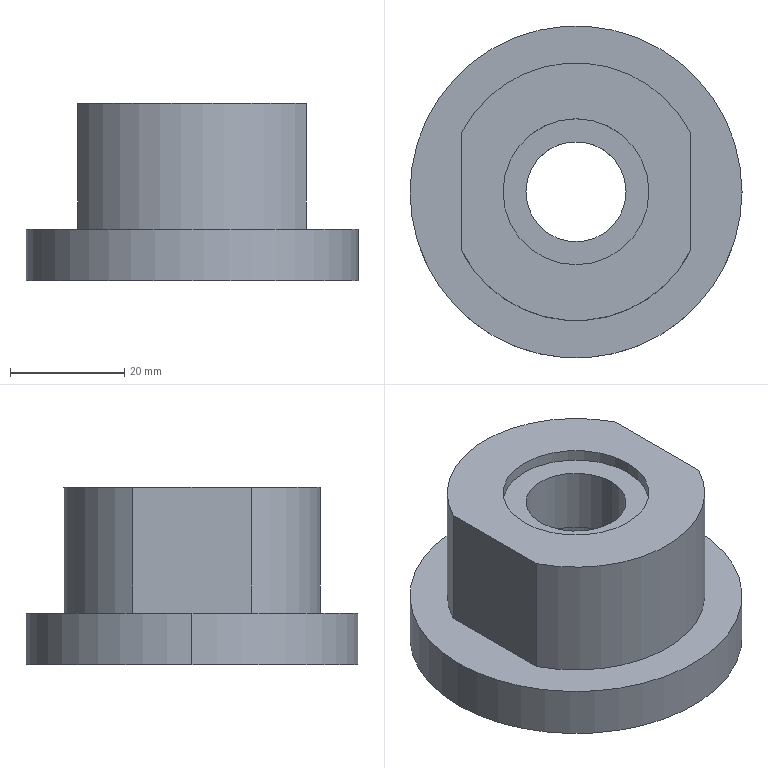Part | SolidWorks | features BaseBody 1 | 1 solid | 17 faces | box 58 x 58 x 31 mm | volume 44160 mm3 | cylinder 10 | plane 7 | commonest cylinder face diameters 17.5 x2 25.5 x2 26 x2 45 x2 58 x2
STEP:
#1=CARTESIAN_POINT('',(13.,0.,17.5));
#2=VERTEX_POINT('',#1);
#3=CARTESIAN_POINT('',(-13.,0.,17.5));
#4=VERTEX_POINT('',#3);
#5=CARTESIAN_POINT('',(0.,0.,17.5));
#6=DIRECTION('',(0.,0.,-1.));
#7=DIRECTION('',(-1.,0.,0.));
#8=AXIS2_PLACEMENT_3D('',#5,#6,#7);
#9=CIRCLE('',#8,13.);
#10=EDGE_CURVE('',#2,#4,#9,.T.);
#11=ORIENTED_EDGE('',*,*,#10,.F.);
#12=CARTESIAN_POINT('',(13.,0.,0.));
#13=VERTEX_POINT('',#12);
#14=CARTESIAN_POINT('',(13.,0.,0.));
#15=DIRECTION('',(0.,0.,-1.));
#16=VECTOR('',#15,1000.);
#17=LINE('',#14,#16);
#18=EDGE_CURVE('',#2,#13,#17,.T.);
#19=ORIENTED_EDGE('',*,*,#18,.T.);
#20=CARTESIAN_POINT('',(-13.,0.,0.));
#21=VERTEX_POINT('',#20);
#22=CARTESIAN_POINT('',(0.,0.,0.));
#23=DIRECTION('',(0.,0.,-1.));
#24=DIRECTION('',(-1.,0.,0.));
#25=AXIS2_PLACEMENT_3D('',#22,#23,#24);
#26=CIRCLE('',#25,13.);
#27=EDGE_CURVE('',#13,#21,#26,.T.);
#28=ORIENTED_EDGE('',*,*,#27,.T.);
#29=CARTESIAN_POINT('',(-13.,0.,0.));
#30=DIRECTION('',(0.,0.,-1.));
#31=VECTOR('',#30,1000.);
#32=LINE('',#29,#31);
#33=EDGE_CURVE('',#4,#21,#32,.T.);
#34=ORIENTED_EDGE('',*,*,#33,.F.);
#35=EDGE_LOOP('',(#11,#19,#28,#34));
#36=FACE_OUTER_BOUND('',#35,.T.);
#37=CARTESIAN_POINT('',(0.,0.,0.));
#38=DIRECTION('',(0.,0.,-1.));
#39=DIRECTION('',(-1.,0.,0.));
#40=AXIS2_PLACEMENT_3D('',#37,#38,#39);
#41=CYLINDRICAL_SURFACE('',#40,13.);
#42=ADVANCED_FACE('',(#36),#41,.F.);
#43=CARTESIAN_POINT('',(-8.75,0.,29.));
#44=VERTEX_POINT('',#43);
#45=CARTESIAN_POINT('',(8.75,0.,29.));
#46=VERTEX_POINT('',#45);
#47=CARTESIAN_POINT('',(0.,0.,29.));
#48=DIRECTION('',(0.,0.,1.));
#49=DIRECTION('',(1.,0.,0.));
#50=AXIS2_PLACEMENT_3D('',#47,#48,#49);
#51=CIRCLE('',#50,8.75);
#52=EDGE_CURVE('',#44,#46,#51,.T.);
#53=ORIENTED_EDGE('',*,*,#52,.T.);
#54=CARTESIAN_POINT('',(8.75,0.,17.5));
#55=VERTEX_POINT('',#54);
#56=CARTESIAN_POINT('',(8.75,0.,0.));
#57=DIRECTION('',(0.,0.,-1.));
#58=VECTOR('',#57,1000.);
#59=LINE('',#56,#58);
#60=EDGE_CURVE('',#46,#55,#59,.T.);
#61=ORIENTED_EDGE('',*,*,#60,.T.);
#62=CARTESIAN_POINT('',(-8.75,0.,17.5));
#63=VERTEX_POINT('',#62);
#64=CARTESIAN_POINT('',(0.,0.,17.5));
#65=DIRECTION('',(0.,0.,-1.));
#66=DIRECTION('',(-1.,0.,0.));
#67=AXIS2_PLACEMENT_3D('',#64,#65,#66);
#68=CIRCLE('',#67,8.75);
#69=EDGE_CURVE('',#55,#63,#68,.T.);
#70=ORIENTED_EDGE('',*,*,#69,.T.);
#71=CARTESIAN_POINT('',(-8.75,0.,0.));
#72=DIRECTION('',(0.,0.,-1.));
#73=VECTOR('',#72,1000.);
#74=LINE('',#71,#73);
#75=EDGE_CURVE('',#44,#63,#74,.T.);
#76=ORIENTED_EDGE('',*,*,#75,.F.);
#77=EDGE_LOOP('',(#53,#61,#70,#76));
#78=FACE_OUTER_BOUND('',#77,.T.);
#79=CARTESIAN_POINT('',(0.,0.,0.));
#80=DIRECTION('',(0.,0.,-1.));
#81=DIRECTION('',(-1.,0.,0.));
#82=AXIS2_PLACEMENT_3D('',#79,#80,#81);
#83=CYLINDRICAL_SURFACE('',#82,8.75);
#84=ADVANCED_FACE('',(#78),#83,.F.);
#85=CARTESIAN_POINT('',(-12.75,0.,29.));
#86=VERTEX_POINT('',#85);
#87=CARTESIAN_POINT('',(12.75,0.,29.));
#88=VERTEX_POINT('',#87);
#89=CARTESIAN_POINT('',(0.,0.,29.));
#90=DIRECTION('',(0.,0.,1.));
#91=DIRECTION('',(1.,0.,0.));
#92=AXIS2_PLACEMENT_3D('',#89,#90,#91);
#93=CIRCLE('',#92,12.75);
#94=EDGE_CURVE('',#86,#88,#93,.T.);
#95=ORIENTED_EDGE('',*,*,#94,.F.);
#96=CARTESIAN_POINT('',(-12.75,0.,31.));
#97=VERTEX_POINT('',#96);
#98=CARTESIAN_POINT('',(-12.75,0.,29.));
#99=DIRECTION('',(0.,0.,1.));
#100=VECTOR('',#99,1000.);
#101=LINE('',#98,#100);
#102=EDGE_CURVE('',#86,#97,#101,.T.);
#103=ORIENTED_EDGE('',*,*,#102,.T.);
#104=CARTESIAN_POINT('',(12.75,0.,31.));
#105=VERTEX_POINT('',#104);
#106=CARTESIAN_POINT('',(0.,0.,31.));
#107=DIRECTION('',(0.,0.,1.));
#108=DIRECTION('',(1.,0.,0.));
#109=AXIS2_PLACEMENT_3D('',#106,#107,#108);
#110=CIRCLE('',#109,12.75);
#111=EDGE_CURVE('',#97,#105,#110,.T.);
#112=ORIENTED_EDGE('',*,*,#111,.T.);
#113=CARTESIAN_POINT('',(12.75,0.,29.));
#114=DIRECTION('',(0.,0.,1.));
#115=VECTOR('',#114,1000.);
#116=LINE('',#113,#115);
#117=EDGE_CURVE('',#88,#105,#116,.T.);
#118=ORIENTED_EDGE('',*,*,#117,.F.);
#119=EDGE_LOOP('',(#95,#103,#112,#118));
#120=FACE_OUTER_BOUND('',#119,.T.);
#121=CARTESIAN_POINT('',(0.,0.,29.));
#122=DIRECTION('',(0.,0.,1.));
#123=DIRECTION('',(1.,0.,0.));
#124=AXIS2_PLACEMENT_3D('',#121,#122,#123);
#125=CYLINDRICAL_SURFACE('',#124,12.75);
#126=ADVANCED_FACE('',(#120),#125,.F.);
#127=CARTESIAN_POINT('',(29.,0.,9.));
#128=VERTEX_POINT('',#127);
#129=CARTESIAN_POINT('',(-29.,0.,9.));
#130=VERTEX_POINT('',#129);
#131=CARTESIAN_POINT('',(0.,0.,9.));
#132=DIRECTION('',(0.,0.,1.));
#133=DIRECTION('',(1.,0.,0.));
#134=AXIS2_PLACEMENT_3D('',#131,#132,#133);
#135=CIRCLE('',#134,29.);
#136=EDGE_CURVE('',#128,#130,#135,.T.);
#137=ORIENTED_EDGE('',*,*,#136,.F.);
#138=CARTESIAN_POINT('',(29.,0.,0.));
#139=VERTEX_POINT('',#138);
#140=CARTESIAN_POINT('',(29.,0.,9.));
#141=DIRECTION('',(0.,0.,-1.));
#142=VECTOR('',#141,1000.);
#143=LINE('',#140,#142);
#144=EDGE_CURVE('',#128,#139,#143,.T.);
#145=ORIENTED_EDGE('',*,*,#144,.T.);
#146=CARTESIAN_POINT('',(-29.,0.,0.));
#147=VERTEX_POINT('',#146);
#148=CARTESIAN_POINT('',(0.,0.,0.));
#149=DIRECTION('',(0.,0.,1.));
#150=DIRECTION('',(1.,0.,0.));
#151=AXIS2_PLACEMENT_3D('',#148,#149,#150);
#152=CIRCLE('',#151,29.);
#153=EDGE_CURVE('',#139,#147,#152,.T.);
#154=ORIENTED_EDGE('',*,*,#153,.T.);
#155=CARTESIAN_POINT('',(-29.,0.,9.));
#156=DIRECTION('',(0.,0.,-1.));
#157=VECTOR('',#156,1000.);
#158=LINE('',#155,#157);
#159=EDGE_CURVE('',#130,#147,#158,.T.);
#160=ORIENTED_EDGE('',*,*,#159,.F.);
#161=EDGE_LOOP('',(#137,#145,#154,#160));
#162=FACE_OUTER_BOUND('',#161,.T.);
#163=CARTESIAN_POINT('',(0.,0.,9.));
#164=DIRECTION('',(0.,0.,-1.));
#165=DIRECTION('',(-1.,0.,0.));
#166=AXIS2_PLACEMENT_3D('',#163,#164,#165);
#167=CYLINDRICAL_SURFACE('',#166,29.);
#168=ADVANCED_FACE('',(#162),#167,.T.);
#169=CARTESIAN_POINT('',(20.,10.308,31.));
#170=VERTEX_POINT('',#169);
#171=CARTESIAN_POINT('',(-20.,10.308,31.));
#172=VERTEX_POINT('',#171);
#173=CARTESIAN_POINT('',(0.,0.,31.));
#174=DIRECTION('',(0.,0.,1.));
#175=DIRECTION('',(1.,0.,0.));
#176=AXIS2_PLACEMENT_3D('',#173,#174,#175);
#177=CIRCLE('',#176,22.5);
#178=EDGE_CURVE('',#170,#172,#177,.T.);
#179=ORIENTED_EDGE('',*,*,#178,.F.);
#180=CARTESIAN_POINT('',(20.,10.308,9.));
#181=VERTEX_POINT('',#180);
#182=CARTESIAN_POINT('',(20.,10.308,31.));
#183=DIRECTION('',(0.,0.,-1.));
#184=VECTOR('',#183,1000.);
#185=LINE('',#182,#184);
#186=EDGE_CURVE('',#170,#181,#185,.T.);
#187=ORIENTED_EDGE('',*,*,#186,.T.);
#188=CARTESIAN_POINT('',(-20.,10.308,9.));
#189=VERTEX_POINT('',#188);
#190=CARTESIAN_POINT('',(0.,0.,9.));
#191=DIRECTION('',(0.,0.,1.));
#192=DIRECTION('',(1.,0.,0.));
#193=AXIS2_PLACEMENT_3D('',#190,#191,#192);
#194=CIRCLE('',#193,22.5);
#195=EDGE_CURVE('',#181,#189,#194,.T.);
#196=ORIENTED_EDGE('',*,*,#195,.T.);
#197=CARTESIAN_POINT('',(-20.,10.308,31.));
#198=DIRECTION('',(0.,0.,1.));
#199=VECTOR('',#198,1000.);
#200=LINE('',#197,#199);
#201=EDGE_CURVE('',#189,#172,#200,.T.);
#202=ORIENTED_EDGE('',*,*,#201,.T.);
#203=EDGE_LOOP('',(#179,#187,#196,#202));
#204=FACE_OUTER_BOUND('',#203,.T.);
#205=CARTESIAN_POINT('',(0.,0.,31.));
#206=DIRECTION('',(0.,0.,-1.));
#207=DIRECTION('',(-1.,0.,0.));
#208=AXIS2_PLACEMENT_3D('',#205,#206,#207);
#209=CYLINDRICAL_SURFACE('',#208,22.5);
#210=ADVANCED_FACE('',(#204),#209,.T.);
#211=ORIENTED_EDGE('',*,*,#144,.F.);
#212=CARTESIAN_POINT('',(0.,0.,9.));
#213=DIRECTION('',(0.,0.,1.));
#214=DIRECTION('',(1.,0.,0.));
#215=AXIS2_PLACEMENT_3D('',#212,#213,#214);
#216=CIRCLE('',#215,29.);
#217=EDGE_CURVE('',#130,#128,#216,.T.);
#218=ORIENTED_EDGE('',*,*,#217,.F.);
#219=ORIENTED_EDGE('',*,*,#159,.T.);
#220=CARTESIAN_POINT('',(0.,0.,0.));
#221=DIRECTION('',(0.,0.,1.));
#222=DIRECTION('',(1.,0.,0.));
#223=AXIS2_PLACEMENT_3D('',#220,#221,#222);
#224=CIRCLE('',#223,29.);
#225=EDGE_CURVE('',#147,#139,#224,.T.);
#226=ORIENTED_EDGE('',*,*,#225,.T.);
#227=EDGE_LOOP('',(#211,#218,#219,#226));
#228=FACE_OUTER_BOUND('',#227,.T.);
#229=CARTESIAN_POINT('',(0.,0.,9.));
#230=DIRECTION('',(0.,0.,-1.));
#231=DIRECTION('',(-1.,0.,0.));
#232=AXIS2_PLACEMENT_3D('',#229,#230,#231);
#233=CYLINDRICAL_SURFACE('',#232,29.);
#234=ADVANCED_FACE('',(#228),#233,.T.);
#235=ORIENTED_EDGE('',*,*,#195,.F.);
#236=CARTESIAN_POINT('',(20.,-10.308,9.));
#237=VERTEX_POINT('',#236);
#238=CARTESIAN_POINT('',(20.,22.361,9.));
#239=DIRECTION('',(0.,-1.,0.));
#240=VECTOR('',#239,1000.);
#241=LINE('',#238,#240);
#242=EDGE_CURVE('',#181,#237,#241,.T.);
#243=ORIENTED_EDGE('',*,*,#242,.T.);
#244=CARTESIAN_POINT('',(-20.,-10.308,9.));
#245=VERTEX_POINT('',#244);
#246=CARTESIAN_POINT('',(0.,0.,9.));
#247=DIRECTION('',(0.,0.,1.));
#248=DIRECTION('',(1.,0.,0.));
#249=AXIS2_PLACEMENT_3D('',#246,#247,#248);
#250=CIRCLE('',#249,22.5);
#251=EDGE_CURVE('',#245,#237,#250,.T.);
#252=ORIENTED_EDGE('',*,*,#251,.F.);
#253=CARTESIAN_POINT('',(-20.,22.361,9.));
#254=DIRECTION('',(0.,1.,0.));
#255=VECTOR('',#254,1000.);
#256=LINE('',#253,#255);
#257=EDGE_CURVE('',#245,#189,#256,.T.);
#258=ORIENTED_EDGE('',*,*,#257,.T.);
#259=EDGE_LOOP('',(#235,#243,#252,#258));
#260=FACE_BOUND('',#259,.T.);
#261=ORIENTED_EDGE('',*,*,#217,.T.);
#262=ORIENTED_EDGE('',*,*,#136,.T.);
#263=EDGE_LOOP('',(#261,#262));
#264=FACE_OUTER_BOUND('',#263,.T.);
#265=CARTESIAN_POINT('',(0.,0.,9.));
#266=DIRECTION('',(0.,0.,1.));
#267=DIRECTION('',(1.,0.,0.));
#268=AXIS2_PLACEMENT_3D('',#265,#266,#267);
#269=PLANE('',#268);
#270=ADVANCED_FACE('',(#260,#264),#269,.T.);
#271=CARTESIAN_POINT('',(0.,0.,0.));
#272=DIRECTION('',(0.,0.,-1.));
#273=DIRECTION('',(-1.,0.,0.));
#274=AXIS2_PLACEMENT_3D('',#271,#272,#273);
#275=CIRCLE('',#274,13.);
#276=EDGE_CURVE('',#21,#13,#275,.T.);
#277=ORIENTED_EDGE('',*,*,#276,.F.);
#278=ORIENTED_EDGE('',*,*,#27,.F.);
#279=EDGE_LOOP('',(#277,#278));
#280=FACE_BOUND('',#279,.T.);
#281=ORIENTED_EDGE('',*,*,#225,.F.);
#282=ORIENTED_EDGE('',*,*,#153,.F.);
#283=EDGE_LOOP('',(#281,#282));
#284=FACE_OUTER_BOUND('',#283,.T.);
#285=CARTESIAN_POINT('',(0.,0.,0.));
#286=DIRECTION('',(0.,0.,1.));
#287=DIRECTION('',(1.,0.,0.));
#288=AXIS2_PLACEMENT_3D('',#285,#286,#287);
#289=PLANE('',#288);
#290=ADVANCED_FACE('',(#280,#284),#289,.F.);
#291=ORIENTED_EDGE('',*,*,#251,.T.);
#292=CARTESIAN_POINT('',(20.,-10.308,31.));
#293=VERTEX_POINT('',#292);
#294=CARTESIAN_POINT('',(20.,-10.308,31.));
#295=DIRECTION('',(0.,0.,1.));
#296=VECTOR('',#295,1000.);
#297=LINE('',#294,#296);
#298=EDGE_CURVE('',#237,#293,#297,.T.);
#299=ORIENTED_EDGE('',*,*,#298,.T.);
#300=CARTESIAN_POINT('',(-20.,-10.308,31.));
#301=VERTEX_POINT('',#300);
#302=CARTESIAN_POINT('',(0.,0.,31.));
#303=DIRECTION('',(0.,0.,1.));
#304=DIRECTION('',(1.,0.,0.));
#305=AXIS2_PLACEMENT_3D('',#302,#303,#304);
#306=CIRCLE('',#305,22.5);
#307=EDGE_CURVE('',#301,#293,#306,.T.);
#308=ORIENTED_EDGE('',*,*,#307,.F.);
#309=CARTESIAN_POINT('',(-20.,-10.308,31.));
#310=DIRECTION('',(0.,0.,-1.));
#311=VECTOR('',#310,1000.);
#312=LINE('',#309,#311);
#313=EDGE_CURVE('',#301,#245,#312,.T.);
#314=ORIENTED_EDGE('',*,*,#313,.T.);
#315=EDGE_LOOP('',(#291,#299,#308,#314));
#316=FACE_OUTER_BOUND('',#315,.T.);
#317=CARTESIAN_POINT('',(0.,0.,31.));
#318=DIRECTION('',(0.,0.,-1.));
#319=DIRECTION('',(-1.,0.,0.));
#320=AXIS2_PLACEMENT_3D('',#317,#318,#319);
#321=CYLINDRICAL_SURFACE('',#320,22.5);
#322=ADVANCED_FACE('',(#316),#321,.T.);
#323=CARTESIAN_POINT('',(20.,0.,31.));
#324=DIRECTION('',(0.,-1.,0.));
#325=VECTOR('',#324,1000.);
#326=LINE('',#323,#325);
#327=EDGE_CURVE('',#170,#293,#326,.T.);
#328=ORIENTED_EDGE('',*,*,#327,.F.);
#329=ORIENTED_EDGE('',*,*,#178,.T.);
#330=CARTESIAN_POINT('',(-20.,0.,31.));
#331=DIRECTION('',(0.,1.,0.));
#332=VECTOR('',#331,1000.);
#333=LINE('',#330,#332);
#334=EDGE_CURVE('',#301,#172,#333,.T.);
#335=ORIENTED_EDGE('',*,*,#334,.F.);
#336=ORIENTED_EDGE('',*,*,#307,.T.);
#337=EDGE_LOOP('',(#328,#329,#335,#336));
#338=FACE_OUTER_BOUND('',#337,.T.);
#339=CARTESIAN_POINT('',(0.,0.,31.));
#340=DIRECTION('',(0.,0.,1.));
#341=DIRECTION('',(1.,0.,0.));
#342=AXIS2_PLACEMENT_3D('',#339,#340,#341);
#343=CIRCLE('',#342,12.75);
#344=EDGE_CURVE('',#105,#97,#343,.T.);
#345=ORIENTED_EDGE('',*,*,#344,.F.);
#346=ORIENTED_EDGE('',*,*,#111,.F.);
#347=EDGE_LOOP('',(#345,#346));
#348=FACE_BOUND('',#347,.T.);
#349=CARTESIAN_POINT('',(0.,0.,31.));
#350=DIRECTION('',(0.,0.,1.));
#351=DIRECTION('',(1.,0.,0.));
#352=AXIS2_PLACEMENT_3D('',#349,#350,#351);
#353=PLANE('',#352);
#354=ADVANCED_FACE('',(#338,#348),#353,.T.);
#355=ORIENTED_EDGE('',*,*,#102,.F.);
#356=CARTESIAN_POINT('',(0.,0.,29.));
#357=DIRECTION('',(0.,0.,1.));
#358=DIRECTION('',(1.,0.,0.));
#359=AXIS2_PLACEMENT_3D('',#356,#357,#358);
#360=CIRCLE('',#359,12.75);
#361=EDGE_CURVE('',#88,#86,#360,.T.);
#362=ORIENTED_EDGE('',*,*,#361,.F.);
#363=ORIENTED_EDGE('',*,*,#117,.T.);
#364=ORIENTED_EDGE('',*,*,#344,.T.);
#365=EDGE_LOOP('',(#355,#362,#363,#364));
#366=FACE_OUTER_BOUND('',#365,.T.);
#367=CARTESIAN_POINT('',(0.,0.,29.));
#368=DIRECTION('',(0.,0.,1.));
#369=DIRECTION('',(1.,0.,0.));
#370=AXIS2_PLACEMENT_3D('',#367,#368,#369);
#371=CYLINDRICAL_SURFACE('',#370,12.75);
#372=ADVANCED_FACE('',(#366),#371,.F.);
#373=ORIENTED_EDGE('',*,*,#52,.F.);
#374=CARTESIAN_POINT('',(0.,0.,29.));
#375=DIRECTION('',(0.,0.,1.));
#376=DIRECTION('',(1.,0.,0.));
#377=AXIS2_PLACEMENT_3D('',#374,#375,#376);
#378=CIRCLE('',#377,8.75);
#379=EDGE_CURVE('',#46,#44,#378,.T.);
#380=ORIENTED_EDGE('',*,*,#379,.F.);
#381=EDGE_LOOP('',(#373,#380));
#382=FACE_BOUND('',#381,.T.);
#383=ORIENTED_EDGE('',*,*,#361,.T.);
#384=ORIENTED_EDGE('',*,*,#94,.T.);
#385=EDGE_LOOP('',(#383,#384));
#386=FACE_OUTER_BOUND('',#385,.T.);
#387=CARTESIAN_POINT('',(0.,0.,29.));
#388=DIRECTION('',(0.,0.,1.));
#389=DIRECTION('',(1.,0.,0.));
#390=AXIS2_PLACEMENT_3D('',#387,#388,#389);
#391=PLANE('',#390);
#392=ADVANCED_FACE('',(#382,#386),#391,.T.);
#393=ORIENTED_EDGE('',*,*,#334,.T.);
#394=ORIENTED_EDGE('',*,*,#201,.F.);
#395=ORIENTED_EDGE('',*,*,#257,.F.);
#396=ORIENTED_EDGE('',*,*,#313,.F.);
#397=EDGE_LOOP('',(#393,#394,#395,#396));
#398=FACE_OUTER_BOUND('',#397,.T.);
#399=CARTESIAN_POINT('',(-20.,22.361,9.));
#400=DIRECTION('',(1.,0.,0.));
#401=DIRECTION('',(0.,0.,-1.));
#402=AXIS2_PLACEMENT_3D('',#399,#400,#401);
#403=PLANE('',#402);
#404=ADVANCED_FACE('',(#398),#403,.F.);
#405=ORIENTED_EDGE('',*,*,#327,.T.);
#406=ORIENTED_EDGE('',*,*,#298,.F.);
#407=ORIENTED_EDGE('',*,*,#242,.F.);
#408=ORIENTED_EDGE('',*,*,#186,.F.);
#409=EDGE_LOOP('',(#405,#406,#407,#408));
#410=FACE_OUTER_BOUND('',#409,.T.);
#411=CARTESIAN_POINT('',(20.,22.361,9.));
#412=DIRECTION('',(-1.,0.,0.));
#413=DIRECTION('',(0.,0.,1.));
#414=AXIS2_PLACEMENT_3D('',#411,#412,#413);
#415=PLANE('',#414);
#416=ADVANCED_FACE('',(#410),#415,.F.);
#417=ORIENTED_EDGE('',*,*,#60,.F.);
#418=ORIENTED_EDGE('',*,*,#379,.T.);
#419=ORIENTED_EDGE('',*,*,#75,.T.);
#420=CARTESIAN_POINT('',(0.,0.,17.5));
#421=DIRECTION('',(0.,0.,-1.));
#422=DIRECTION('',(-1.,0.,0.));
#423=AXIS2_PLACEMENT_3D('',#420,#421,#422);
#424=CIRCLE('',#423,8.75);
#425=EDGE_CURVE('',#63,#55,#424,.T.);
#426=ORIENTED_EDGE('',*,*,#425,.T.);
#427=EDGE_LOOP('',(#417,#418,#419,#426));
#428=FACE_OUTER_BOUND('',#427,.T.);
#429=CARTESIAN_POINT('',(0.,0.,0.));
#430=DIRECTION('',(0.,0.,-1.));
#431=DIRECTION('',(-1.,0.,0.));
#432=AXIS2_PLACEMENT_3D('',#429,#430,#431);
#433=CYLINDRICAL_SURFACE('',#432,8.75);
#434=ADVANCED_FACE('',(#428),#433,.F.);
#435=ORIENTED_EDGE('',*,*,#425,.F.);
#436=ORIENTED_EDGE('',*,*,#69,.F.);
#437=EDGE_LOOP('',(#435,#436));
#438=FACE_BOUND('',#437,.T.);
#439=CARTESIAN_POINT('',(0.,0.,17.5));
#440=DIRECTION('',(0.,0.,-1.));
#441=DIRECTION('',(-1.,0.,0.));
#442=AXIS2_PLACEMENT_3D('',#439,#440,#441);
#443=CIRCLE('',#442,13.);
#444=EDGE_CURVE('',#4,#2,#443,.T.);
#445=ORIENTED_EDGE('',*,*,#444,.T.);
#446=ORIENTED_EDGE('',*,*,#10,.T.);
#447=EDGE_LOOP('',(#445,#446));
#448=FACE_OUTER_BOUND('',#447,.T.);
#449=CARTESIAN_POINT('',(8.75,0.,17.5));
#450=DIRECTION('',(0.,0.,1.));
#451=DIRECTION('',(1.,0.,0.));
#452=AXIS2_PLACEMENT_3D('',#449,#450,#451);
#453=PLANE('',#452);
#454=ADVANCED_FACE('',(#438,#448),#453,.F.);
#455=ORIENTED_EDGE('',*,*,#18,.F.);
#456=ORIENTED_EDGE('',*,*,#444,.F.);
#457=ORIENTED_EDGE('',*,*,#33,.T.);
#458=ORIENTED_EDGE('',*,*,#276,.T.);
#459=EDGE_LOOP('',(#455,#456,#457,#458));
#460=FACE_OUTER_BOUND('',#459,.T.);
#461=CARTESIAN_POINT('',(0.,0.,0.));
#462=DIRECTION('',(0.,0.,-1.));
#463=DIRECTION('',(-1.,0.,0.));
#464=AXIS2_PLACEMENT_3D('',#461,#462,#463);
#465=CYLINDRICAL_SURFACE('',#464,13.);
#466=ADVANCED_FACE('',(#460),#465,.F.);
#467=CLOSED_SHELL('',(#42,#84,#126,#168,#210,#234,#270,#290,#322,#354,#372,#392,#404,#416,#434,#454,#466));
#468=MANIFOLD_SOLID_BREP('',#467);
#469=CARTESIAN_POINT('',(0.,0.,0.));
#470=DIRECTION('',(0.,0.,1.));
#471=DIRECTION('',(1.,0.,0.));
#472=AXIS2_PLACEMENT_3D('',#469,#470,#471);
#473=(LENGTH_UNIT()NAMED_UNIT(*)SI_UNIT(.MILLI.,.METRE.));
#474=UNCERTAINTY_MEASURE_WITH_UNIT(LENGTH_MEASURE(0.00001),#473,'','');
#475=(NAMED_UNIT(*)PLANE_ANGLE_UNIT()SI_UNIT($,.RADIAN.));
#476=(NAMED_UNIT(*)SI_UNIT($,.STERADIAN.)SOLID_ANGLE_UNIT());
#477=(GEOMETRIC_REPRESENTATION_CONTEXT(3)GLOBAL_UNCERTAINTY_ASSIGNED_CONTEXT((#474))GLOBAL_UNIT_ASSIGNED_CONTEXT((#473,#475,#476))REPRESENTATION_CONTEXT('',''));
#478=ADVANCED_BREP_SHAPE_REPRESENTATION('',(#468,#472),#477);